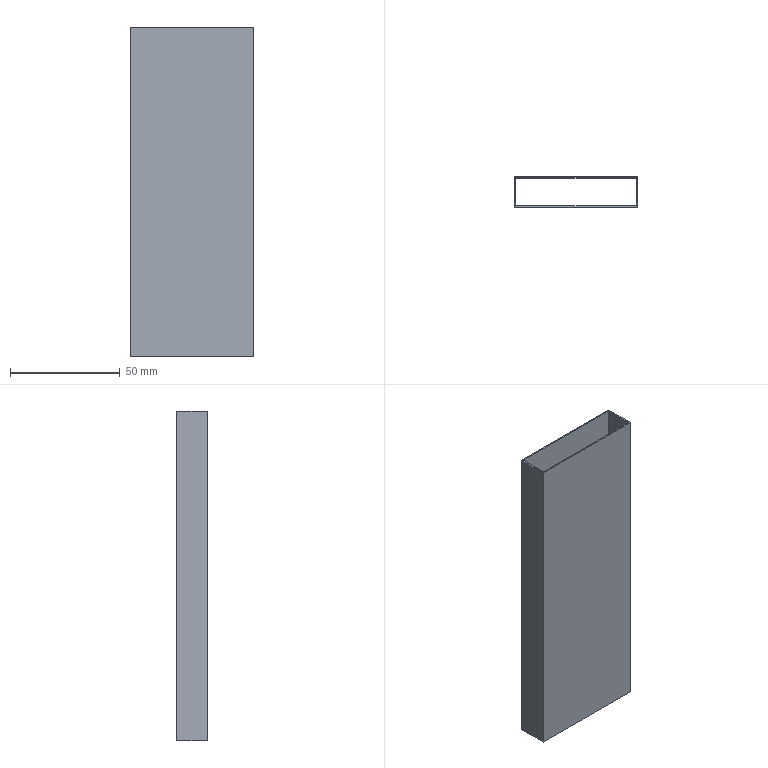Part | STEP file | Plastic bag | 1 solid | 10 faces | box 56 x 14 x 150 mm | volume 10350 mm3 | plane 10
STEP:
#1=CARTESIAN_POINT('',(0.,0.,0.));
#2=DIRECTION('',(0.,0.,1.));
#3=DIRECTION('',(1.,0.,0.));
#4=AXIS2_PLACEMENT_3D('',#1,#2,#3);
#5=CARTESIAN_POINT('',(28.,-7.,150.));
#6=VERTEX_POINT('',#5);
#7=CARTESIAN_POINT('',(28.,7.,150.));
#8=VERTEX_POINT('',#7);
#9=CARTESIAN_POINT('',(28.,-7.,150.));
#10=DIRECTION('',(0.,1.,0.));
#11=VECTOR('',#10,1.);
#12=LINE('',#9,#11);
#13=CARTESIAN_POINT('',(0.,0.,150.));
#14=DIRECTION('',(0.,0.,-1.));
#15=DIRECTION('',(-1.,0.,0.));
#16=AXIS2_PLACEMENT_3D('',#13,#14,#15);
#17=PLANE('',#16);
#18=CARTESIAN_POINT('',(-28.,-7.));
#19=DIRECTION('',(0.,1.));
#20=VECTOR('',#19,1.);
#21=LINE('',#18,#20);
#22=(GEOMETRIC_REPRESENTATION_CONTEXT(2)PARAMETRIC_REPRESENTATION_CONTEXT()REPRESENTATION_CONTEXT('',''));
#23=DEFINITIONAL_REPRESENTATION('',(#21),#22);
#24=PCURVE('',#17,#23);
#25=CARTESIAN_POINT('',(28.,-7.,150.));
#26=DIRECTION('',(-1.,0.,0.));
#27=DIRECTION('',(0.,0.,1.));
#28=AXIS2_PLACEMENT_3D('',#25,#26,#27);
#29=PLANE('',#28);
#30=CARTESIAN_POINT('',(0.,0.));
#31=DIRECTION('',(0.,1.));
#32=VECTOR('',#31,1.);
#33=LINE('',#30,#32);
#34=(GEOMETRIC_REPRESENTATION_CONTEXT(2)PARAMETRIC_REPRESENTATION_CONTEXT()REPRESENTATION_CONTEXT('',''));
#35=DEFINITIONAL_REPRESENTATION('',(#33),#34);
#36=PCURVE('',#29,#35);
#37=SURFACE_CURVE('',#12,(#24,#36),.PCURVE_S1.);
#38=EDGE_CURVE('',#6,#8,#37,.T.);
#39=ORIENTED_EDGE('',*,*,#38,.T.);
#40=CARTESIAN_POINT('',(-28.,7.,150.));
#41=VERTEX_POINT('',#40);
#42=CARTESIAN_POINT('',(-28.,7.,150.));
#43=DIRECTION('',(-1.,0.,0.));
#44=VECTOR('',#43,1.);
#45=LINE('',#42,#44);
#46=CARTESIAN_POINT('',(28.,7.));
#47=DIRECTION('',(1.,0.));
#48=VECTOR('',#47,1.);
#49=LINE('',#46,#48);
#50=(GEOMETRIC_REPRESENTATION_CONTEXT(2)PARAMETRIC_REPRESENTATION_CONTEXT()REPRESENTATION_CONTEXT('',''));
#51=DEFINITIONAL_REPRESENTATION('',(#49),#50);
#52=PCURVE('',#17,#51);
#53=CARTESIAN_POINT('',(-28.,7.,150.));
#54=DIRECTION('',(0.,-1.,0.));
#55=DIRECTION('',(0.,0.,-1.));
#56=AXIS2_PLACEMENT_3D('',#53,#54,#55);
#57=PLANE('',#56);
#58=CARTESIAN_POINT('',(0.,0.));
#59=DIRECTION('',(0.,-1.));
#60=VECTOR('',#59,1.);
#61=LINE('',#58,#60);
#62=(GEOMETRIC_REPRESENTATION_CONTEXT(2)PARAMETRIC_REPRESENTATION_CONTEXT()REPRESENTATION_CONTEXT('',''));
#63=DEFINITIONAL_REPRESENTATION('',(#61),#62);
#64=PCURVE('',#57,#63);
#65=SURFACE_CURVE('',#45,(#52,#64),.PCURVE_S1.);
#66=EDGE_CURVE('',#8,#41,#65,.T.);
#67=ORIENTED_EDGE('',*,*,#66,.T.);
#68=CARTESIAN_POINT('',(-28.,-7.,150.));
#69=VERTEX_POINT('',#68);
#70=CARTESIAN_POINT('',(-28.,-7.,150.));
#71=DIRECTION('',(0.,-1.,0.));
#72=VECTOR('',#71,1.);
#73=LINE('',#70,#72);
#74=CARTESIAN_POINT('',(28.,-7.));
#75=DIRECTION('',(0.,-1.));
#76=VECTOR('',#75,1.);
#77=LINE('',#74,#76);
#78=(GEOMETRIC_REPRESENTATION_CONTEXT(2)PARAMETRIC_REPRESENTATION_CONTEXT()REPRESENTATION_CONTEXT('',''));
#79=DEFINITIONAL_REPRESENTATION('',(#77),#78);
#80=PCURVE('',#17,#79);
#81=CARTESIAN_POINT('',(-28.,-7.,150.));
#82=DIRECTION('',(1.,0.,0.));
#83=DIRECTION('',(0.,0.,-1.));
#84=AXIS2_PLACEMENT_3D('',#81,#82,#83);
#85=PLANE('',#84);
#86=CARTESIAN_POINT('',(0.,0.));
#87=DIRECTION('',(0.,-1.));
#88=VECTOR('',#87,1.);
#89=LINE('',#86,#88);
#90=(GEOMETRIC_REPRESENTATION_CONTEXT(2)PARAMETRIC_REPRESENTATION_CONTEXT()REPRESENTATION_CONTEXT('',''));
#91=DEFINITIONAL_REPRESENTATION('',(#89),#90);
#92=PCURVE('',#85,#91);
#93=SURFACE_CURVE('',#73,(#80,#92),.PCURVE_S1.);
#94=EDGE_CURVE('',#41,#69,#93,.T.);
#95=ORIENTED_EDGE('',*,*,#94,.T.);
#96=CARTESIAN_POINT('',(-28.,-7.,150.));
#97=DIRECTION('',(1.,0.,0.));
#98=VECTOR('',#97,1.);
#99=LINE('',#96,#98);
#100=CARTESIAN_POINT('',(28.,-7.));
#101=DIRECTION('',(-1.,0.));
#102=VECTOR('',#101,1.);
#103=LINE('',#100,#102);
#104=(GEOMETRIC_REPRESENTATION_CONTEXT(2)PARAMETRIC_REPRESENTATION_CONTEXT()REPRESENTATION_CONTEXT('',''));
#105=DEFINITIONAL_REPRESENTATION('',(#103),#104);
#106=PCURVE('',#17,#105);
#107=CARTESIAN_POINT('',(-28.,-7.,150.));
#108=DIRECTION('',(0.,1.,0.));
#109=DIRECTION('',(0.,0.,1.));
#110=AXIS2_PLACEMENT_3D('',#107,#108,#109);
#111=PLANE('',#110);
#112=CARTESIAN_POINT('',(0.,0.));
#113=DIRECTION('',(0.,1.));
#114=VECTOR('',#113,1.);
#115=LINE('',#112,#114);
#116=(GEOMETRIC_REPRESENTATION_CONTEXT(2)PARAMETRIC_REPRESENTATION_CONTEXT()REPRESENTATION_CONTEXT('',''));
#117=DEFINITIONAL_REPRESENTATION('',(#115),#116);
#118=PCURVE('',#111,#117);
#119=SURFACE_CURVE('',#99,(#106,#118),.PCURVE_S1.);
#120=EDGE_CURVE('',#69,#6,#119,.T.);
#121=ORIENTED_EDGE('',*,*,#120,.T.);
#122=EDGE_LOOP('',(#39,#67,#95,#121));
#123=FACE_BOUND('',#122,.T.);
#124=CARTESIAN_POINT('',(-27.5,6.5,150.));
#125=VERTEX_POINT('',#124);
#126=CARTESIAN_POINT('',(-27.5,-6.5,150.));
#127=VERTEX_POINT('',#126);
#128=CARTESIAN_POINT('',(-27.5,-6.5,150.));
#129=DIRECTION('',(0.,-1.,0.));
#130=VECTOR('',#129,1.);
#131=LINE('',#128,#130);
#132=CARTESIAN_POINT('',(27.5,-6.5));
#133=DIRECTION('',(0.,-1.));
#134=VECTOR('',#133,1.);
#135=LINE('',#132,#134);
#136=(GEOMETRIC_REPRESENTATION_CONTEXT(2)PARAMETRIC_REPRESENTATION_CONTEXT()REPRESENTATION_CONTEXT('',''));
#137=DEFINITIONAL_REPRESENTATION('',(#135),#136);
#138=PCURVE('',#17,#137);
#139=CARTESIAN_POINT('',(-27.5,-6.5,150.));
#140=DIRECTION('',(1.,0.,0.));
#141=DIRECTION('',(0.,0.,-1.));
#142=AXIS2_PLACEMENT_3D('',#139,#140,#141);
#143=PLANE('',#142);
#144=CARTESIAN_POINT('',(0.,0.));
#145=DIRECTION('',(0.,-1.));
#146=VECTOR('',#145,1.);
#147=LINE('',#144,#146);
#148=(GEOMETRIC_REPRESENTATION_CONTEXT(2)PARAMETRIC_REPRESENTATION_CONTEXT()REPRESENTATION_CONTEXT('',''));
#149=DEFINITIONAL_REPRESENTATION('',(#147),#148);
#150=PCURVE('',#143,#149);
#151=SURFACE_CURVE('',#131,(#138,#150),.PCURVE_S1.);
#152=EDGE_CURVE('',#125,#127,#151,.T.);
#153=ORIENTED_EDGE('',*,*,#152,.F.);
#154=CARTESIAN_POINT('',(27.5,6.5,150.));
#155=VERTEX_POINT('',#154);
#156=CARTESIAN_POINT('',(-27.5,6.5,150.));
#157=DIRECTION('',(-1.,0.,0.));
#158=VECTOR('',#157,1.);
#159=LINE('',#156,#158);
#160=CARTESIAN_POINT('',(27.5,6.5));
#161=DIRECTION('',(1.,0.));
#162=VECTOR('',#161,1.);
#163=LINE('',#160,#162);
#164=(GEOMETRIC_REPRESENTATION_CONTEXT(2)PARAMETRIC_REPRESENTATION_CONTEXT()REPRESENTATION_CONTEXT('',''));
#165=DEFINITIONAL_REPRESENTATION('',(#163),#164);
#166=PCURVE('',#17,#165);
#167=CARTESIAN_POINT('',(-27.5,6.5,150.));
#168=DIRECTION('',(0.,-1.,0.));
#169=DIRECTION('',(0.,0.,-1.));
#170=AXIS2_PLACEMENT_3D('',#167,#168,#169);
#171=PLANE('',#170);
#172=CARTESIAN_POINT('',(0.,0.));
#173=DIRECTION('',(0.,-1.));
#174=VECTOR('',#173,1.);
#175=LINE('',#172,#174);
#176=(GEOMETRIC_REPRESENTATION_CONTEXT(2)PARAMETRIC_REPRESENTATION_CONTEXT()REPRESENTATION_CONTEXT('',''));
#177=DEFINITIONAL_REPRESENTATION('',(#175),#176);
#178=PCURVE('',#171,#177);
#179=SURFACE_CURVE('',#159,(#166,#178),.PCURVE_S1.);
#180=EDGE_CURVE('',#155,#125,#179,.T.);
#181=ORIENTED_EDGE('',*,*,#180,.F.);
#182=CARTESIAN_POINT('',(27.5,-6.5,150.));
#183=VERTEX_POINT('',#182);
#184=CARTESIAN_POINT('',(27.5,-6.5,150.));
#185=DIRECTION('',(0.,1.,0.));
#186=VECTOR('',#185,1.);
#187=LINE('',#184,#186);
#188=CARTESIAN_POINT('',(-27.5,-6.5));
#189=DIRECTION('',(0.,1.));
#190=VECTOR('',#189,1.);
#191=LINE('',#188,#190);
#192=(GEOMETRIC_REPRESENTATION_CONTEXT(2)PARAMETRIC_REPRESENTATION_CONTEXT()REPRESENTATION_CONTEXT('',''));
#193=DEFINITIONAL_REPRESENTATION('',(#191),#192);
#194=PCURVE('',#17,#193);
#195=CARTESIAN_POINT('',(27.5,-6.5,150.));
#196=DIRECTION('',(-1.,0.,0.));
#197=DIRECTION('',(0.,0.,1.));
#198=AXIS2_PLACEMENT_3D('',#195,#196,#197);
#199=PLANE('',#198);
#200=CARTESIAN_POINT('',(0.,0.));
#201=DIRECTION('',(0.,1.));
#202=VECTOR('',#201,1.);
#203=LINE('',#200,#202);
#204=(GEOMETRIC_REPRESENTATION_CONTEXT(2)PARAMETRIC_REPRESENTATION_CONTEXT()REPRESENTATION_CONTEXT('',''));
#205=DEFINITIONAL_REPRESENTATION('',(#203),#204);
#206=PCURVE('',#199,#205);
#207=SURFACE_CURVE('',#187,(#194,#206),.PCURVE_S1.);
#208=EDGE_CURVE('',#183,#155,#207,.T.);
#209=ORIENTED_EDGE('',*,*,#208,.F.);
#210=CARTESIAN_POINT('',(-27.5,-6.5,150.));
#211=DIRECTION('',(1.,0.,0.));
#212=VECTOR('',#211,1.);
#213=LINE('',#210,#212);
#214=CARTESIAN_POINT('',(27.5,-6.5));
#215=DIRECTION('',(-1.,0.));
#216=VECTOR('',#215,1.);
#217=LINE('',#214,#216);
#218=(GEOMETRIC_REPRESENTATION_CONTEXT(2)PARAMETRIC_REPRESENTATION_CONTEXT()REPRESENTATION_CONTEXT('',''));
#219=DEFINITIONAL_REPRESENTATION('',(#217),#218);
#220=PCURVE('',#17,#219);
#221=CARTESIAN_POINT('',(-27.5,-6.5,150.));
#222=DIRECTION('',(0.,1.,0.));
#223=DIRECTION('',(0.,0.,1.));
#224=AXIS2_PLACEMENT_3D('',#221,#222,#223);
#225=PLANE('',#224);
#226=CARTESIAN_POINT('',(0.,0.));
#227=DIRECTION('',(0.,1.));
#228=VECTOR('',#227,1.);
#229=LINE('',#226,#228);
#230=(GEOMETRIC_REPRESENTATION_CONTEXT(2)PARAMETRIC_REPRESENTATION_CONTEXT()REPRESENTATION_CONTEXT('',''));
#231=DEFINITIONAL_REPRESENTATION('',(#229),#230);
#232=PCURVE('',#225,#231);
#233=SURFACE_CURVE('',#213,(#220,#232),.PCURVE_S1.);
#234=EDGE_CURVE('',#127,#183,#233,.T.);
#235=ORIENTED_EDGE('',*,*,#234,.F.);
#236=EDGE_LOOP('',(#153,#181,#209,#235));
#237=FACE_BOUND('',#236,.T.);
#238=ADVANCED_FACE('',(#123,#237),#17,.F.);
#239=CARTESIAN_POINT('',(28.,-7.,0.));
#240=VERTEX_POINT('',#239);
#241=CARTESIAN_POINT('',(28.,7.,0.));
#242=VERTEX_POINT('',#241);
#243=CARTESIAN_POINT('',(28.,-7.,0.));
#244=DIRECTION('',(0.,1.,0.));
#245=VECTOR('',#244,1.);
#246=LINE('',#243,#245);
#247=CARTESIAN_POINT('',(0.,0.,0.));
#248=DIRECTION('',(0.,0.,-1.));
#249=DIRECTION('',(-1.,0.,0.));
#250=AXIS2_PLACEMENT_3D('',#247,#248,#249);
#251=PLANE('',#250);
#252=CARTESIAN_POINT('',(-28.,-7.));
#253=DIRECTION('',(0.,1.));
#254=VECTOR('',#253,1.);
#255=LINE('',#252,#254);
#256=(GEOMETRIC_REPRESENTATION_CONTEXT(2)PARAMETRIC_REPRESENTATION_CONTEXT()REPRESENTATION_CONTEXT('',''));
#257=DEFINITIONAL_REPRESENTATION('',(#255),#256);
#258=PCURVE('',#251,#257);
#259=CARTESIAN_POINT('',(-150.,0.));
#260=DIRECTION('',(0.,1.));
#261=VECTOR('',#260,1.);
#262=LINE('',#259,#261);
#263=(GEOMETRIC_REPRESENTATION_CONTEXT(2)PARAMETRIC_REPRESENTATION_CONTEXT()REPRESENTATION_CONTEXT('',''));
#264=DEFINITIONAL_REPRESENTATION('',(#262),#263);
#265=PCURVE('',#29,#264);
#266=SURFACE_CURVE('',#246,(#258,#265),.PCURVE_S1.);
#267=EDGE_CURVE('',#240,#242,#266,.T.);
#268=ORIENTED_EDGE('',*,*,#267,.F.);
#269=CARTESIAN_POINT('',(-28.,-7.,0.));
#270=VERTEX_POINT('',#269);
#271=CARTESIAN_POINT('',(-28.,-7.,0.));
#272=DIRECTION('',(1.,0.,0.));
#273=VECTOR('',#272,1.);
#274=LINE('',#271,#273);
#275=CARTESIAN_POINT('',(28.,-7.));
#276=DIRECTION('',(-1.,0.));
#277=VECTOR('',#276,1.);
#278=LINE('',#275,#277);
#279=(GEOMETRIC_REPRESENTATION_CONTEXT(2)PARAMETRIC_REPRESENTATION_CONTEXT()REPRESENTATION_CONTEXT('',''));
#280=DEFINITIONAL_REPRESENTATION('',(#278),#279);
#281=PCURVE('',#251,#280);
#282=CARTESIAN_POINT('',(-150.,0.));
#283=DIRECTION('',(0.,1.));
#284=VECTOR('',#283,1.);
#285=LINE('',#282,#284);
#286=(GEOMETRIC_REPRESENTATION_CONTEXT(2)PARAMETRIC_REPRESENTATION_CONTEXT()REPRESENTATION_CONTEXT('',''));
#287=DEFINITIONAL_REPRESENTATION('',(#285),#286);
#288=PCURVE('',#111,#287);
#289=SURFACE_CURVE('',#274,(#281,#288),.PCURVE_S1.);
#290=EDGE_CURVE('',#270,#240,#289,.T.);
#291=ORIENTED_EDGE('',*,*,#290,.F.);
#292=CARTESIAN_POINT('',(-28.,7.,0.));
#293=VERTEX_POINT('',#292);
#294=CARTESIAN_POINT('',(-28.,-7.,0.));
#295=DIRECTION('',(0.,-1.,0.));
#296=VECTOR('',#295,1.);
#297=LINE('',#294,#296);
#298=CARTESIAN_POINT('',(28.,-7.));
#299=DIRECTION('',(0.,-1.));
#300=VECTOR('',#299,1.);
#301=LINE('',#298,#300);
#302=(GEOMETRIC_REPRESENTATION_CONTEXT(2)PARAMETRIC_REPRESENTATION_CONTEXT()REPRESENTATION_CONTEXT('',''));
#303=DEFINITIONAL_REPRESENTATION('',(#301),#302);
#304=PCURVE('',#251,#303);
#305=CARTESIAN_POINT('',(150.,0.));
#306=DIRECTION('',(0.,-1.));
#307=VECTOR('',#306,1.);
#308=LINE('',#305,#307);
#309=(GEOMETRIC_REPRESENTATION_CONTEXT(2)PARAMETRIC_REPRESENTATION_CONTEXT()REPRESENTATION_CONTEXT('',''));
#310=DEFINITIONAL_REPRESENTATION('',(#308),#309);
#311=PCURVE('',#85,#310);
#312=SURFACE_CURVE('',#297,(#304,#311),.PCURVE_S1.);
#313=EDGE_CURVE('',#293,#270,#312,.T.);
#314=ORIENTED_EDGE('',*,*,#313,.F.);
#315=CARTESIAN_POINT('',(-28.,7.,0.));
#316=DIRECTION('',(-1.,0.,0.));
#317=VECTOR('',#316,1.);
#318=LINE('',#315,#317);
#319=CARTESIAN_POINT('',(28.,7.));
#320=DIRECTION('',(1.,0.));
#321=VECTOR('',#320,1.);
#322=LINE('',#319,#321);
#323=(GEOMETRIC_REPRESENTATION_CONTEXT(2)PARAMETRIC_REPRESENTATION_CONTEXT()REPRESENTATION_CONTEXT('',''));
#324=DEFINITIONAL_REPRESENTATION('',(#322),#323);
#325=PCURVE('',#251,#324);
#326=CARTESIAN_POINT('',(150.,0.));
#327=DIRECTION('',(0.,-1.));
#328=VECTOR('',#327,1.);
#329=LINE('',#326,#328);
#330=(GEOMETRIC_REPRESENTATION_CONTEXT(2)PARAMETRIC_REPRESENTATION_CONTEXT()REPRESENTATION_CONTEXT('',''));
#331=DEFINITIONAL_REPRESENTATION('',(#329),#330);
#332=PCURVE('',#57,#331);
#333=SURFACE_CURVE('',#318,(#325,#332),.PCURVE_S1.);
#334=EDGE_CURVE('',#242,#293,#333,.T.);
#335=ORIENTED_EDGE('',*,*,#334,.F.);
#336=EDGE_LOOP('',(#268,#291,#314,#335));
#337=FACE_BOUND('',#336,.T.);
#338=CARTESIAN_POINT('',(27.5,6.5,0.));
#339=VERTEX_POINT('',#338);
#340=CARTESIAN_POINT('',(-27.5,6.5,0.));
#341=VERTEX_POINT('',#340);
#342=CARTESIAN_POINT('',(-27.5,6.5,0.));
#343=DIRECTION('',(-1.,0.,0.));
#344=VECTOR('',#343,1.);
#345=LINE('',#342,#344);
#346=CARTESIAN_POINT('',(27.5,6.5));
#347=DIRECTION('',(1.,0.));
#348=VECTOR('',#347,1.);
#349=LINE('',#346,#348);
#350=(GEOMETRIC_REPRESENTATION_CONTEXT(2)PARAMETRIC_REPRESENTATION_CONTEXT()REPRESENTATION_CONTEXT('',''));
#351=DEFINITIONAL_REPRESENTATION('',(#349),#350);
#352=PCURVE('',#251,#351);
#353=CARTESIAN_POINT('',(150.,0.));
#354=DIRECTION('',(0.,-1.));
#355=VECTOR('',#354,1.);
#356=LINE('',#353,#355);
#357=(GEOMETRIC_REPRESENTATION_CONTEXT(2)PARAMETRIC_REPRESENTATION_CONTEXT()REPRESENTATION_CONTEXT('',''));
#358=DEFINITIONAL_REPRESENTATION('',(#356),#357);
#359=PCURVE('',#171,#358);
#360=SURFACE_CURVE('',#345,(#352,#359),.PCURVE_S1.);
#361=EDGE_CURVE('',#339,#341,#360,.T.);
#362=ORIENTED_EDGE('',*,*,#361,.T.);
#363=CARTESIAN_POINT('',(-27.5,-6.5,0.));
#364=VERTEX_POINT('',#363);
#365=CARTESIAN_POINT('',(-27.5,-6.5,0.));
#366=DIRECTION('',(0.,-1.,0.));
#367=VECTOR('',#366,1.);
#368=LINE('',#365,#367);
#369=CARTESIAN_POINT('',(27.5,-6.5));
#370=DIRECTION('',(0.,-1.));
#371=VECTOR('',#370,1.);
#372=LINE('',#369,#371);
#373=(GEOMETRIC_REPRESENTATION_CONTEXT(2)PARAMETRIC_REPRESENTATION_CONTEXT()REPRESENTATION_CONTEXT('',''));
#374=DEFINITIONAL_REPRESENTATION('',(#372),#373);
#375=PCURVE('',#251,#374);
#376=CARTESIAN_POINT('',(150.,0.));
#377=DIRECTION('',(0.,-1.));
#378=VECTOR('',#377,1.);
#379=LINE('',#376,#378);
#380=(GEOMETRIC_REPRESENTATION_CONTEXT(2)PARAMETRIC_REPRESENTATION_CONTEXT()REPRESENTATION_CONTEXT('',''));
#381=DEFINITIONAL_REPRESENTATION('',(#379),#380);
#382=PCURVE('',#143,#381);
#383=SURFACE_CURVE('',#368,(#375,#382),.PCURVE_S1.);
#384=EDGE_CURVE('',#341,#364,#383,.T.);
#385=ORIENTED_EDGE('',*,*,#384,.T.);
#386=CARTESIAN_POINT('',(27.5,-6.5,0.));
#387=VERTEX_POINT('',#386);
#388=CARTESIAN_POINT('',(-27.5,-6.5,0.));
#389=DIRECTION('',(1.,0.,0.));
#390=VECTOR('',#389,1.);
#391=LINE('',#388,#390);
#392=CARTESIAN_POINT('',(27.5,-6.5));
#393=DIRECTION('',(-1.,0.));
#394=VECTOR('',#393,1.);
#395=LINE('',#392,#394);
#396=(GEOMETRIC_REPRESENTATION_CONTEXT(2)PARAMETRIC_REPRESENTATION_CONTEXT()REPRESENTATION_CONTEXT('',''));
#397=DEFINITIONAL_REPRESENTATION('',(#395),#396);
#398=PCURVE('',#251,#397);
#399=CARTESIAN_POINT('',(-150.,0.));
#400=DIRECTION('',(0.,1.));
#401=VECTOR('',#400,1.);
#402=LINE('',#399,#401);
#403=(GEOMETRIC_REPRESENTATION_CONTEXT(2)PARAMETRIC_REPRESENTATION_CONTEXT()REPRESENTATION_CONTEXT('',''));
#404=DEFINITIONAL_REPRESENTATION('',(#402),#403);
#405=PCURVE('',#225,#404);
#406=SURFACE_CURVE('',#391,(#398,#405),.PCURVE_S1.);
#407=EDGE_CURVE('',#364,#387,#406,.T.);
#408=ORIENTED_EDGE('',*,*,#407,.T.);
#409=CARTESIAN_POINT('',(27.5,-6.5,0.));
#410=DIRECTION('',(0.,1.,0.));
#411=VECTOR('',#410,1.);
#412=LINE('',#409,#411);
#413=CARTESIAN_POINT('',(-27.5,-6.5));
#414=DIRECTION('',(0.,1.));
#415=VECTOR('',#414,1.);
#416=LINE('',#413,#415);
#417=(GEOMETRIC_REPRESENTATION_CONTEXT(2)PARAMETRIC_REPRESENTATION_CONTEXT()REPRESENTATION_CONTEXT('',''));
#418=DEFINITIONAL_REPRESENTATION('',(#416),#417);
#419=PCURVE('',#251,#418);
#420=CARTESIAN_POINT('',(-150.,0.));
#421=DIRECTION('',(0.,1.));
#422=VECTOR('',#421,1.);
#423=LINE('',#420,#422);
#424=(GEOMETRIC_REPRESENTATION_CONTEXT(2)PARAMETRIC_REPRESENTATION_CONTEXT()REPRESENTATION_CONTEXT('',''));
#425=DEFINITIONAL_REPRESENTATION('',(#423),#424);
#426=PCURVE('',#199,#425);
#427=SURFACE_CURVE('',#412,(#419,#426),.PCURVE_S1.);
#428=EDGE_CURVE('',#387,#339,#427,.T.);
#429=ORIENTED_EDGE('',*,*,#428,.T.);
#430=EDGE_LOOP('',(#362,#385,#408,#429));
#431=FACE_BOUND('',#430,.T.);
#432=ADVANCED_FACE('',(#337,#431),#251,.T.);
#433=ORIENTED_EDGE('',*,*,#267,.T.);
#434=CARTESIAN_POINT('',(28.,7.,150.));
#435=DIRECTION('',(0.,0.,-1.));
#436=VECTOR('',#435,1.);
#437=LINE('',#434,#436);
#438=CARTESIAN_POINT('',(0.,14.));
#439=DIRECTION('',(-1.,0.));
#440=VECTOR('',#439,1.);
#441=LINE('',#438,#440);
#442=(GEOMETRIC_REPRESENTATION_CONTEXT(2)PARAMETRIC_REPRESENTATION_CONTEXT()REPRESENTATION_CONTEXT('',''));
#443=DEFINITIONAL_REPRESENTATION('',(#441),#442);
#444=PCURVE('',#29,#443);
#445=CARTESIAN_POINT('',(0.,56.));
#446=DIRECTION('',(1.,0.));
#447=VECTOR('',#446,1.);
#448=LINE('',#445,#447);
#449=(GEOMETRIC_REPRESENTATION_CONTEXT(2)PARAMETRIC_REPRESENTATION_CONTEXT()REPRESENTATION_CONTEXT('',''));
#450=DEFINITIONAL_REPRESENTATION('',(#448),#449);
#451=PCURVE('',#57,#450);
#452=SURFACE_CURVE('',#437,(#444,#451),.PCURVE_S1.);
#453=EDGE_CURVE('',#8,#242,#452,.T.);
#454=ORIENTED_EDGE('',*,*,#453,.F.);
#455=ORIENTED_EDGE('',*,*,#38,.F.);
#456=CARTESIAN_POINT('',(28.,-7.,150.));
#457=DIRECTION('',(0.,0.,-1.));
#458=VECTOR('',#457,1.);
#459=LINE('',#456,#458);
#460=CARTESIAN_POINT('',(0.,0.));
#461=DIRECTION('',(-1.,0.));
#462=VECTOR('',#461,1.);
#463=LINE('',#460,#462);
#464=(GEOMETRIC_REPRESENTATION_CONTEXT(2)PARAMETRIC_REPRESENTATION_CONTEXT()REPRESENTATION_CONTEXT('',''));
#465=DEFINITIONAL_REPRESENTATION('',(#463),#464);
#466=PCURVE('',#29,#465);
#467=CARTESIAN_POINT('',(0.,56.));
#468=DIRECTION('',(-1.,0.));
#469=VECTOR('',#468,1.);
#470=LINE('',#467,#469);
#471=(GEOMETRIC_REPRESENTATION_CONTEXT(2)PARAMETRIC_REPRESENTATION_CONTEXT()REPRESENTATION_CONTEXT('',''));
#472=DEFINITIONAL_REPRESENTATION('',(#470),#471);
#473=PCURVE('',#111,#472);
#474=SURFACE_CURVE('',#459,(#466,#473),.PCURVE_S1.);
#475=EDGE_CURVE('',#6,#240,#474,.T.);
#476=ORIENTED_EDGE('',*,*,#475,.T.);
#477=EDGE_LOOP('',(#433,#454,#455,#476));
#478=FACE_BOUND('',#477,.T.);
#479=ADVANCED_FACE('',(#478),#29,.F.);
#480=ORIENTED_EDGE('',*,*,#334,.T.);
#481=CARTESIAN_POINT('',(-28.,7.,150.));
#482=DIRECTION('',(0.,0.,-1.));
#483=VECTOR('',#482,1.);
#484=LINE('',#481,#483);
#485=CARTESIAN_POINT('',(0.,0.));
#486=DIRECTION('',(1.,0.));
#487=VECTOR('',#486,1.);
#488=LINE('',#485,#487);
#489=(GEOMETRIC_REPRESENTATION_CONTEXT(2)PARAMETRIC_REPRESENTATION_CONTEXT()REPRESENTATION_CONTEXT('',''));
#490=DEFINITIONAL_REPRESENTATION('',(#488),#489);
#491=PCURVE('',#57,#490);
#492=CARTESIAN_POINT('',(0.,14.));
#493=DIRECTION('',(1.,0.));
#494=VECTOR('',#493,1.);
#495=LINE('',#492,#494);
#496=(GEOMETRIC_REPRESENTATION_CONTEXT(2)PARAMETRIC_REPRESENTATION_CONTEXT()REPRESENTATION_CONTEXT('',''));
#497=DEFINITIONAL_REPRESENTATION('',(#495),#496);
#498=PCURVE('',#85,#497);
#499=SURFACE_CURVE('',#484,(#491,#498),.PCURVE_S1.);
#500=EDGE_CURVE('',#41,#293,#499,.T.);
#501=ORIENTED_EDGE('',*,*,#500,.F.);
#502=ORIENTED_EDGE('',*,*,#66,.F.);
#503=ORIENTED_EDGE('',*,*,#453,.T.);
#504=EDGE_LOOP('',(#480,#501,#502,#503));
#505=FACE_BOUND('',#504,.T.);
#506=ADVANCED_FACE('',(#505),#57,.F.);
#507=ORIENTED_EDGE('',*,*,#313,.T.);
#508=CARTESIAN_POINT('',(-28.,-7.,150.));
#509=DIRECTION('',(0.,0.,-1.));
#510=VECTOR('',#509,1.);
#511=LINE('',#508,#510);
#512=CARTESIAN_POINT('',(0.,0.));
#513=DIRECTION('',(1.,0.));
#514=VECTOR('',#513,1.);
#515=LINE('',#512,#514);
#516=(GEOMETRIC_REPRESENTATION_CONTEXT(2)PARAMETRIC_REPRESENTATION_CONTEXT()REPRESENTATION_CONTEXT('',''));
#517=DEFINITIONAL_REPRESENTATION('',(#515),#516);
#518=PCURVE('',#85,#517);
#519=CARTESIAN_POINT('',(0.,0.));
#520=DIRECTION('',(-1.,0.));
#521=VECTOR('',#520,1.);
#522=LINE('',#519,#521);
#523=(GEOMETRIC_REPRESENTATION_CONTEXT(2)PARAMETRIC_REPRESENTATION_CONTEXT()REPRESENTATION_CONTEXT('',''));
#524=DEFINITIONAL_REPRESENTATION('',(#522),#523);
#525=PCURVE('',#111,#524);
#526=SURFACE_CURVE('',#511,(#518,#525),.PCURVE_S1.);
#527=EDGE_CURVE('',#69,#270,#526,.T.);
#528=ORIENTED_EDGE('',*,*,#527,.F.);
#529=ORIENTED_EDGE('',*,*,#94,.F.);
#530=ORIENTED_EDGE('',*,*,#500,.T.);
#531=EDGE_LOOP('',(#507,#528,#529,#530));
#532=FACE_BOUND('',#531,.T.);
#533=ADVANCED_FACE('',(#532),#85,.F.);
#534=ORIENTED_EDGE('',*,*,#290,.T.);
#535=ORIENTED_EDGE('',*,*,#475,.F.);
#536=ORIENTED_EDGE('',*,*,#120,.F.);
#537=ORIENTED_EDGE('',*,*,#527,.T.);
#538=EDGE_LOOP('',(#534,#535,#536,#537));
#539=FACE_BOUND('',#538,.T.);
#540=ADVANCED_FACE('',(#539),#111,.F.);
#541=ORIENTED_EDGE('',*,*,#384,.F.);
#542=CARTESIAN_POINT('',(-27.5,6.5,150.));
#543=DIRECTION('',(0.,0.,-1.));
#544=VECTOR('',#543,1.);
#545=LINE('',#542,#544);
#546=CARTESIAN_POINT('',(0.,13.));
#547=DIRECTION('',(1.,0.));
#548=VECTOR('',#547,1.);
#549=LINE('',#546,#548);
#550=(GEOMETRIC_REPRESENTATION_CONTEXT(2)PARAMETRIC_REPRESENTATION_CONTEXT()REPRESENTATION_CONTEXT('',''));
#551=DEFINITIONAL_REPRESENTATION('',(#549),#550);
#552=PCURVE('',#143,#551);
#553=CARTESIAN_POINT('',(0.,0.));
#554=DIRECTION('',(1.,0.));
#555=VECTOR('',#554,1.);
#556=LINE('',#553,#555);
#557=(GEOMETRIC_REPRESENTATION_CONTEXT(2)PARAMETRIC_REPRESENTATION_CONTEXT()REPRESENTATION_CONTEXT('',''));
#558=DEFINITIONAL_REPRESENTATION('',(#556),#557);
#559=PCURVE('',#171,#558);
#560=SURFACE_CURVE('',#545,(#552,#559),.PCURVE_S1.);
#561=EDGE_CURVE('',#125,#341,#560,.T.);
#562=ORIENTED_EDGE('',*,*,#561,.F.);
#563=ORIENTED_EDGE('',*,*,#152,.T.);
#564=CARTESIAN_POINT('',(-27.5,-6.5,150.));
#565=DIRECTION('',(0.,0.,-1.));
#566=VECTOR('',#565,1.);
#567=LINE('',#564,#566);
#568=CARTESIAN_POINT('',(0.,0.));
#569=DIRECTION('',(1.,0.));
#570=VECTOR('',#569,1.);
#571=LINE('',#568,#570);
#572=(GEOMETRIC_REPRESENTATION_CONTEXT(2)PARAMETRIC_REPRESENTATION_CONTEXT()REPRESENTATION_CONTEXT('',''));
#573=DEFINITIONAL_REPRESENTATION('',(#571),#572);
#574=PCURVE('',#143,#573);
#575=CARTESIAN_POINT('',(0.,0.));
#576=DIRECTION('',(-1.,0.));
#577=VECTOR('',#576,1.);
#578=LINE('',#575,#577);
#579=(GEOMETRIC_REPRESENTATION_CONTEXT(2)PARAMETRIC_REPRESENTATION_CONTEXT()REPRESENTATION_CONTEXT('',''));
#580=DEFINITIONAL_REPRESENTATION('',(#578),#579);
#581=PCURVE('',#225,#580);
#582=SURFACE_CURVE('',#567,(#574,#581),.PCURVE_S1.);
#583=EDGE_CURVE('',#127,#364,#582,.T.);
#584=ORIENTED_EDGE('',*,*,#583,.T.);
#585=EDGE_LOOP('',(#541,#562,#563,#584));
#586=FACE_BOUND('',#585,.T.);
#587=ADVANCED_FACE('',(#586),#143,.T.);
#588=ORIENTED_EDGE('',*,*,#407,.F.);
#589=ORIENTED_EDGE('',*,*,#583,.F.);
#590=ORIENTED_EDGE('',*,*,#234,.T.);
#591=CARTESIAN_POINT('',(27.5,-6.5,150.));
#592=DIRECTION('',(0.,0.,-1.));
#593=VECTOR('',#592,1.);
#594=LINE('',#591,#593);
#595=CARTESIAN_POINT('',(0.,55.));
#596=DIRECTION('',(-1.,0.));
#597=VECTOR('',#596,1.);
#598=LINE('',#595,#597);
#599=(GEOMETRIC_REPRESENTATION_CONTEXT(2)PARAMETRIC_REPRESENTATION_CONTEXT()REPRESENTATION_CONTEXT('',''));
#600=DEFINITIONAL_REPRESENTATION('',(#598),#599);
#601=PCURVE('',#225,#600);
#602=CARTESIAN_POINT('',(0.,0.));
#603=DIRECTION('',(-1.,0.));
#604=VECTOR('',#603,1.);
#605=LINE('',#602,#604);
#606=(GEOMETRIC_REPRESENTATION_CONTEXT(2)PARAMETRIC_REPRESENTATION_CONTEXT()REPRESENTATION_CONTEXT('',''));
#607=DEFINITIONAL_REPRESENTATION('',(#605),#606);
#608=PCURVE('',#199,#607);
#609=SURFACE_CURVE('',#594,(#601,#608),.PCURVE_S1.);
#610=EDGE_CURVE('',#183,#387,#609,.T.);
#611=ORIENTED_EDGE('',*,*,#610,.T.);
#612=EDGE_LOOP('',(#588,#589,#590,#611));
#613=FACE_BOUND('',#612,.T.);
#614=ADVANCED_FACE('',(#613),#225,.T.);
#615=ORIENTED_EDGE('',*,*,#428,.F.);
#616=ORIENTED_EDGE('',*,*,#610,.F.);
#617=ORIENTED_EDGE('',*,*,#208,.T.);
#618=CARTESIAN_POINT('',(27.5,6.5,150.));
#619=DIRECTION('',(0.,0.,-1.));
#620=VECTOR('',#619,1.);
#621=LINE('',#618,#620);
#622=CARTESIAN_POINT('',(0.,13.));
#623=DIRECTION('',(-1.,0.));
#624=VECTOR('',#623,1.);
#625=LINE('',#622,#624);
#626=(GEOMETRIC_REPRESENTATION_CONTEXT(2)PARAMETRIC_REPRESENTATION_CONTEXT()REPRESENTATION_CONTEXT('',''));
#627=DEFINITIONAL_REPRESENTATION('',(#625),#626);
#628=PCURVE('',#199,#627);
#629=CARTESIAN_POINT('',(0.,55.));
#630=DIRECTION('',(1.,0.));
#631=VECTOR('',#630,1.);
#632=LINE('',#629,#631);
#633=(GEOMETRIC_REPRESENTATION_CONTEXT(2)PARAMETRIC_REPRESENTATION_CONTEXT()REPRESENTATION_CONTEXT('',''));
#634=DEFINITIONAL_REPRESENTATION('',(#632),#633);
#635=PCURVE('',#171,#634);
#636=SURFACE_CURVE('',#621,(#628,#635),.PCURVE_S1.);
#637=EDGE_CURVE('',#155,#339,#636,.T.);
#638=ORIENTED_EDGE('',*,*,#637,.T.);
#639=EDGE_LOOP('',(#615,#616,#617,#638));
#640=FACE_BOUND('',#639,.T.);
#641=ADVANCED_FACE('',(#640),#199,.T.);
#642=ORIENTED_EDGE('',*,*,#361,.F.);
#643=ORIENTED_EDGE('',*,*,#637,.F.);
#644=ORIENTED_EDGE('',*,*,#180,.T.);
#645=ORIENTED_EDGE('',*,*,#561,.T.);
#646=EDGE_LOOP('',(#642,#643,#644,#645));
#647=FACE_BOUND('',#646,.T.);
#648=ADVANCED_FACE('',(#647),#171,.T.);
#649=CLOSED_SHELL('',(#238,#432,#479,#506,#533,#540,#587,#614,#641,#648));
#650=MANIFOLD_SOLID_BREP('',#649);
#651=(LENGTH_UNIT()NAMED_UNIT(*)SI_UNIT(.MILLI.,.METRE.));
#652=UNCERTAINTY_MEASURE_WITH_UNIT(LENGTH_MEASURE(0.0000001),#651,'','');
#653=(NAMED_UNIT(*)PLANE_ANGLE_UNIT()SI_UNIT($,.RADIAN.));
#654=(NAMED_UNIT(*)SI_UNIT($,.STERADIAN.)SOLID_ANGLE_UNIT());
#655=(GEOMETRIC_REPRESENTATION_CONTEXT(3)GLOBAL_UNCERTAINTY_ASSIGNED_CONTEXT((#652))GLOBAL_UNIT_ASSIGNED_CONTEXT((#651,#653,#654))REPRESENTATION_CONTEXT('',''));
#656=ADVANCED_BREP_SHAPE_REPRESENTATION('',(#4,#650),#655);